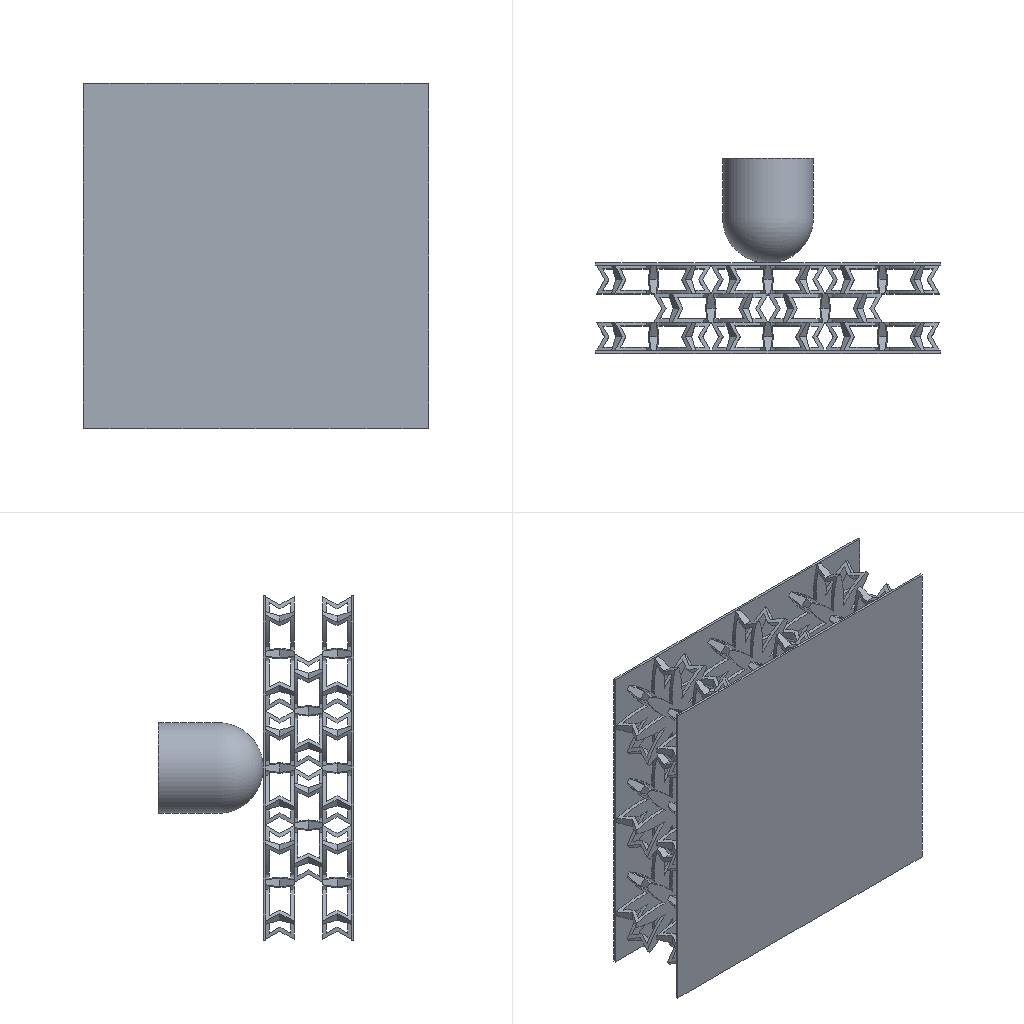Simulation study | abaqus
Set-up summary:
category,name,step,type,value,unit,region
solver,abaqus
solver,version,,,Abaqus/Explicit 2020
units,not stated in the deck,,not stated
analysis,deck,,transient,transient
load_step,Step-1,Step-1,transient,nlgeom=True
contact,interactions,,,general=1 pairs=0 ties=0
load_step,requested,,,1
mesh,nodes,,,32318
mesh,elements,,,67672
element_type,C3D4,,solid,58663
element_type,C3D8R,,solid,9009
load,load commands in deck,,count,1
bc,support commands in deck,,count,6
material,MATERIAL-1,,in results
material,S,,in results
check,setup vs results,,match,"per instance, exact: element labels, types and connectivity; labels of the nodes the elements use; coordinates of those nodes at SINGLE_PRECISION in 2 of 2 instance(s)"
Abaqus input file, long lists of numbers shortened:
*Heading
** Job name: Job-1 Model name: Model-1
** Generated by: Abaqus/CAE 2020
*Preprint, echo=NO, model=NO, history=NO, contact=NO
**
** PARTS
**
*Part, name=Part-2
*Node
      1,    -35.999,   24.641,   81.136
      2,   -32.864,   24.641,   84.271
** (22180 more lines like these left out)
*Element, type=C3D4
    1, 11965, 15032, 11964, 12012
    2,  9913, 22030,  8141,  1979
** (58661 more lines like these left out)
*Nset, nset=Set-4, generate
     1,  22182,      1
*Elset, elset=Set-4, generate
     1,  58663,      1
** Section: Section-1
*Solid Section, elset=Set-4, material=Material-1
,
*End Part
**
*Part, name=rig
*Node
      1,   18.634,  -3.961,           0.
      2,   18.118,  -5.887,           0.
** (10134 more lines like these left out)
*Element, type=C3D8R
   1,    80,   615,   570,    56,   804,  1339,  1294,   780
   2,    56,   571,   621,    57,   780,  1295,  1345,   781
** (9007 more lines like these left out)
*Nset, nset=Set-1, generate
     1,  10136,      1
*Elset, elset=Set-1, generate
    1,  9009,     1
** Section: s
*Solid Section, elset=Set-1, material=s
,
*End Part
**
**
** ASSEMBLY
**
*Assembly, name=Assembly
**
*Instance, name=Part-2-1, part=Part-2
*End Instance
**
*Instance, name=rig-1, part=rig
    0.2722,    50.691,          48.
*End Instance
**
*Node
      1,  0.2722,   75.691,          48.
*Nset, nset=Set-1, instance=Part-2-1
  2409,  2410,  2411,  2412,  9189,  9190,  9191,  9192,  9193,  9194,  9195,  9196,  9197,  9198,  9199,  9200
  9201,  9202,  9203,  9204,  9205,  9206,  9207,  9208,  9209,  9210,  9211,  9212,  9213,  9214,  9215,  9216
** (149 more lines like these left out)
*Elset, elset=Set-1, instance=Part-2-1
    35,   123,   205,   492,   810,   816,   828,   834,   835,   842,   848,   861,   866,   878,   932,   933
   943,   968,   982,   994,  1032,  1033,  1048,  1074,  1075,  1086,  1094,  1104,  1183,  1185,  1191,  1193
** (286 more lines like these left out)
*Nset, nset=Set-3
 1,
*Nset, nset=Set-4
 1,
*Nset, nset=Set-7
 1,
*Nset, nset=b_Set-5, instance=rig-1, generate
     1,  10136,      1
*Elset, elset=b_Set-5, instance=rig-1, generate
    1,  9009,     1
*Nset, nset=_PickedSet196, internal
 1,
** Constraint: Constraint-1
*Rigid Body, ref node=_PickedSet196, elset=b_Set-5
*Element, type=MASS, elset=Set-4_Inertia-1_
1, 1
*Mass, elset=Set-4_Inertia-1_
0.0013,
*End Assembly
*Amplitude, name=Amp-1
             0.,           1.086,         0.00025,          12.722,          0.0005,           4.423,         0.00075,           6.729
          0.001,          12.492,         0.00125,           5.115,          0.0015,          10.878,         0.00175,          12.953
          0.002,           8.342,         0.00225,           15.95,          0.0025,          13.644,         0.00275,          -2.262
          0.003,          10.417,         0.00325,           3.271,          0.0035,           0.504,         0.00375,           8.342
          0.004,          13.875,         0.00425,           8.573,          0.0045,           9.726,         0.00475,           8.573
          0.005,          -1.109,         0.00525,           11.57,          0.0055,            3.04,         0.00575,          -2.262
          0.006,           8.803,         0.00625,          19.408,          0.0065,          16.641,         0.00675,          12.031
          0.007,           9.264,         0.00725,          12.031,          0.0075,            7.19,         0.00775,          14.336
          0.008,           6.959,         0.00825,          -7.333,          0.0085,           6.729,         0.00875,           1.888
          0.009,          30.473,         0.00925,          61.363,          0.0095,         106.777,         0.00975,         142.048
           0.01,         171.555,         0.01025,         219.966,          0.0105,          94.329,         0.01075,         148.963
          0.011,         102.858,         0.01125,         119.687,          0.0115,         117.842,         0.01175,          98.709
          0.012,         110.466,         0.01225,         107.238,          0.0125,         136.284,         0.01275,         116.229
          0.013,         154.035,         0.01325,         182.851,          0.0135,         172.016,         0.01375,         237.255
          0.014,         238.177,         0.01425,         286.818,          0.0145,         123.144,         0.01475,          95.251
          0.015,         175.243,         0.01525,         107.469,          0.0155,          156.34,         0.01575,         149.424
          0.016,         175.243,         0.01625,         163.026,          0.0165,         114.154,         0.01675,         167.406
          0.017,         151.038,         0.01725,         166.944,          0.0175,         133.288,         0.01775,         151.269
          0.018,         133.057,         0.01825,         163.026,          0.0185,         204.751,         0.01875,            187.
          0.019,         238.638,         0.01925,         255.236,          0.0195,         277.136,         0.01975,         255.928
           0.02,          309.64,         0.02025,         319.783,          0.0205,         306.413,         0.02075,         300.189
          0.021,          344.68,         0.02125,         368.885,          0.0215,         394.474,         0.02175,         387.789
          0.022,         128.908,         0.02225,         207.056,          0.0225,         175.243,         0.02275,         150.116
          0.023,         205.903,         0.02325,          164.87,          0.0235,         189.997,         0.02375,         170.402
          0.024,          178.24,         0.02425,         169.019,          0.0245,         196.913,         0.02475,         181.237
          0.025,         206.595,         0.02525,         207.978,          0.0255,         158.415,         0.02575,          235.18
          0.026,         215.355,         0.02625,         266.071,          0.0265,         235.872,         0.02675,         270.451
          0.027,         251.778,         0.02725,         329.466,          0.0275,          309.64,         0.02775,         337.303
          0.028,         357.359,         0.02825,         358.512,          0.0285,         389.633,         0.02875,         409.228
          0.029,         424.903,         0.02925,          471.47,          0.0295,         487.607,         0.02975,         503.513
           0.03,         525.182,         0.03025,         541.319,          0.0305,         568.521,         0.03075,           581.2
          0.031,         591.343,         0.03125,         580.278,          0.0315,         582.583,         0.03175,         618.315
          0.032,         617.393,         0.03225,         630.763,          0.0325,         599.181,         0.03275,         618.545
          0.033,         610.938,         0.03325,         592.957,          0.0335,         570.365,         0.03375,         538.092
          0.034,         529.562,         0.03425,         492.909,          0.0345,          458.33,         0.03475,          436.43
          0.035,           384.1,         0.03525,         349.982,          0.0355,         325.316,         0.03575,         297.883
          0.036,         273.909,         0.03625,         241.635,          0.0365,         207.748,         0.03675,         189.075
          0.037,         181.698,         0.03725,         161.642,          0.0375,         141.587,         0.03775,          116.92
          0.038,         113.462,         0.03825,          84.877,          0.0385,          55.139,         0.03875,          71.507
          0.039,          53.987,         0.03925,          52.834,          0.0395,          19.177,         0.03975,          64.821
** (11 more lines like these left out)
**
** MATERIALS
**
*Material, name=Material-1
*Density
 1.2e-09,
*Elastic
2800., 0.34
*Material, name=s
*Density
 7.8e-09,
*Elastic
210000., 0.3
**
** INTERACTION PROPERTIES
**
*Surface Interaction, name=IntProp-1
*Friction
 0.2,
*Surface Behavior, pressure-overclosure=HARD
** ----------------------------------------------------------------
**
** STEP: Step-1
**
*Step, name=Step-1, nlgeom=YES
*Dynamic, Explicit
, 0.05
*Bulk Viscosity
0.06, 1.2
** Mass Scaling: Semi-Automatic
**               Whole Model
*Fixed Mass Scaling, factor=50.
**
** BOUNDARY CONDITIONS
**
** Name: BC-1 Type: 对称/反对称/完全固定
*Boundary
Set-1, ENCASTRE
** Name: BC-2 Type: 位移/转角
*Boundary
Set-3, 1, 1
Set-3, 3, 3
Set-3, 4, 4
Set-3, 5, 5
Set-3, 6, 6
**
** LOADS
**
** Name: Load-1   Type: Concentrated force
*Cload, amplitude=Amp-1
Set-7, 2, -1.
**
** INTERACTIONS
**
** Interaction: Int-1
*Contact, op=NEW
*Contact Inclusions, ALL EXTERIOR
*Contact Property Assignment
 ,  , IntProp-1
**
** OUTPUT REQUESTS
**
*Restart, write, number interval=1, time marks=NO
**
** FIELD OUTPUT: F-Output-1
**
*Output, field, number interval=50
*Node Output
A, CF, RF, RM, RT, U, V
*Element Output, directions=YES
E, EVF, LE, MISES, MISESMAX, MISESONLY, PE, PEEQ, PEEQVAVG, PEVAVG, PRESSONLY, S, SEQUT, SF, SVAVG, YIELDPOT
*Contact Output
CDISP, CFORCE, CSTRESS, FSLIP, FSLIPR, PPRESS
**
** HISTORY OUTPUT: H-Output-1
**
*Output, history, variable=PRESELECT, time interval=2.5e-05
**
** HISTORY OUTPUT: H-Output-2
**
*Output, history, time interval=1e-05
*Node Output, nset=Set-3
CF2, U2
*End Step
Results summary:
result,step,Step-1,completed,increments=29749 time=0.05/0.05
result,analysis,,,transient
result,last_loadstep,,,1
result,analysis steps,,count,1
result,primary field,,,U
result,reaction total,,FX,-0.4855,model units
result,reaction total,,FY,520.64,model units
result,reaction total,,FZ,2.417,model units